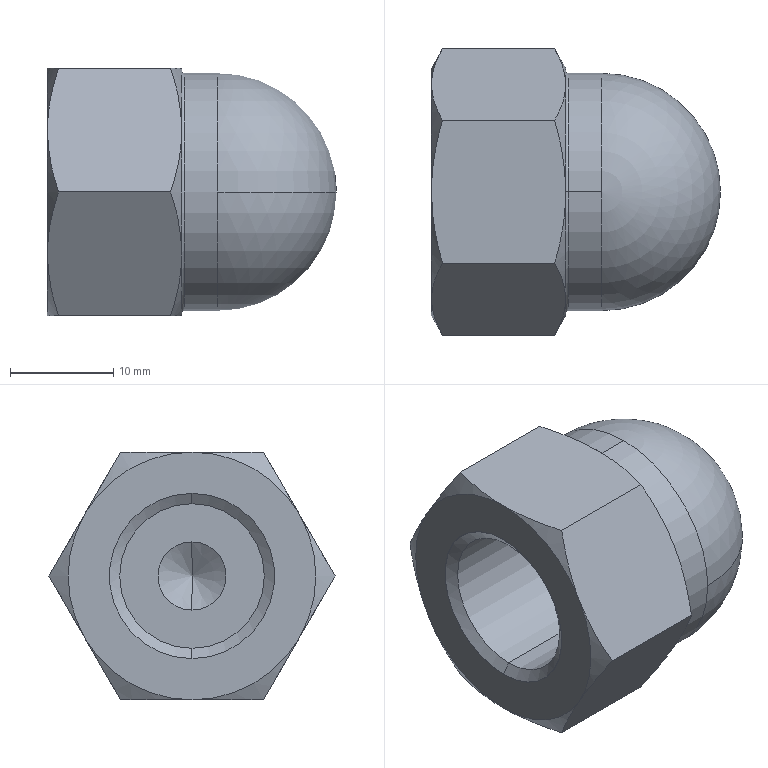Part | SolidWorks | features RevCut 5, Extrusion 1, Fillet 1, LPattern 1, Revolution 1 | 1 solid | 39 faces | box 28 x 27.713 x 24 mm | volume 7401 mm3 | cone 18 | plane 9 | cylinder 8 | torus 2 | sphere 2 | commonest cylinder face diameters 14 x2 16 x2 16.16 x2 23 x2